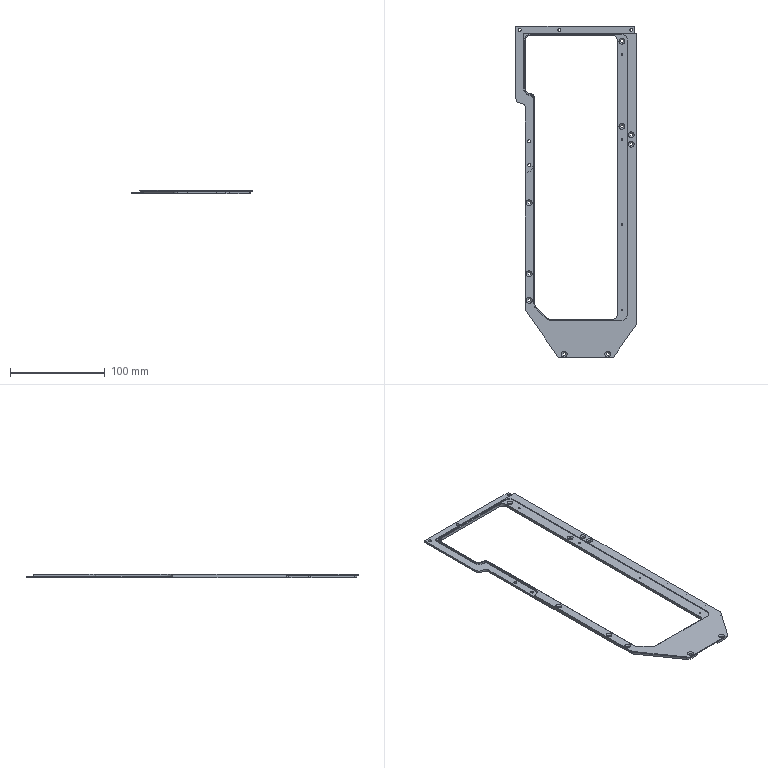NC program | NX | posted with a generic post | part box 127 x 351 x 4 mm
Whole program:
N10 G17 G21 G94 G90
(SPOT_FACING , TOOL : CHAMFER_D8-90DEG)
N12 T01 M6
N14 G54
N16 G17 G0 G90 X153.952 Y40.61 S2500 M3
N18 G43 Z20. H1
N20 G94 G82 G99 Z-2.5 F200. P200 R6.
N22 Y-28.911
N24 G80
N26 G0 X153.952 Y-28.911 Z20.
(SPOT_FACING_COPY_1 , TOOL : CHAMFER_D8-90DEG)
N28 X-8. Y49.5
N30 G82 Z-1.5 F200. P200 R6.
N32 X-83.
N34 X-111.
N36 X-168. Y12.5
N38 Y-33.5
N40 X54. Y-58.5
N42 X163. Y-48.5
N44 X175. Y59.5
N46 Y-58.5
N48 G80
N50 G0 X175. Y-58.5 Z20.
N52 M5
(SPOT_FACING_COPY_1_COPY , TOOL : D2.5)
N54 T15 M6
N56 G54
N58 G17 G0 G90 X-8. Y49.5 S3000 M3
N60 G43 Z20. H15
N62 G94 G83 G99 Z-10. F200. Q2. R6.
N64 X-83.
N66 X-111.
N68 X-168. Y12.5
N70 Y-33.5
N72 X54. Y-58.5
N74 X175. Y59.5
N76 Y-58.5
N78 G80
N80 G0 X175. Y-58.5 Z20.
N82 M5
(SPOT_FACING_COPY , TOOL : DRILL_D4.3-54-83)
N84 T10 M6
N86 G54
N88 G17 G0 G90 X153.952 Y40.61 S3000 M3
N90 G43 Z20. H10
N92 G94 G83 G99 Z-15. F200. Q2. R6.
N94 Y-28.911
N96 G80
N98 G0 X153.952 Y-28.911 Z20.
N100 M5
(PLANAR_MILL_10 , TOOL : D6-18-D6-50-3T-ROUGH)
N102 T03 M6
N104 G54
N106 G17 G0 G90 X-99.149 Y-4.194 S4500 M3
N108 G43 Z20. H3
N110 Z2.
N112 G94 G1 X-99.14 Y-4.178 Z1.999 F800.
N114 X-99.028 Y-3.328 Z1.969
N116 X-99.285 Y-2.51 Z1.939
N118 X-99.865 Y-1.878 Z1.91
N120 X-100.657 Y-1.55 Z1.88
N122 X-101.343 Z1.856
N124 X-102.135 Y-1.878 Z1.826
N126 X-102.715 Y-2.51 Z1.796
N128 X-102.972 Y-3.328 Z1.766
N130 X-102.86 Y-4.178 Z1.736
N132 X-102.517 Y-4.772 Z1.712
N134 X-101.99 Y-5.215 Z1.688
N136 X-101.343 Y-5.45 Z1.664
N138 X-100.657 Z1.64
N140 X-100.01 Y-5.215 Z1.616
N142 X-99.483 Y-4.772 Z1.592
N144 X-99.14 Y-4.178 Z1.568
N146 X-99.028 Y-3.328 Z1.538
N148 X-99.285 Y-2.51 Z1.508
N150 X-99.865 Y-1.878 Z1.478
N152 X-100.657 Y-1.55 Z1.448
N154 X-101.343 Z1.424
N156 X-102.135 Y-1.878 Z1.394
N158 X-102.715 Y-2.51 Z1.364
N160 X-102.972 Y-3.328 Z1.334
N162 X-102.86 Y-4.178 Z1.304
N164 X-102.517 Y-4.772 Z1.28
N166 X-101.99 Y-5.215 Z1.256
N168 X-101.343 Y-5.45 Z1.232
N170 X-100.657 Z1.208
N172 X-100.01 Y-5.215 Z1.184
N174 X-99.483 Y-4.772 Z1.16
N176 X-99.14 Y-4.178 Z1.136
N178 X-99.028 Y-3.328 Z1.106
N180 X-99.285 Y-2.51 Z1.076
N182 X-99.865 Y-1.878 Z1.046
N184 X-100.657 Y-1.55 Z1.017
N186 X-101.343 Z0.993
N188 X-102.135 Y-1.878 Z0.963
N190 X-102.715 Y-2.51 Z0.933
N192 X-102.972 Y-3.328 Z0.903
N194 X-102.86 Y-4.178 Z0.873
N196 X-102.517 Y-4.772 Z0.849
N198 X-101.99 Y-5.215 Z0.825
N200 X-101.343 Y-5.45 Z0.801
N202 X-100.657 Z0.777
N204 X-100.01 Y-5.215 Z0.753
N206 X-99.483 Y-4.772 Z0.729
N208 X-99.14 Y-4.178 Z0.705
N210 X-99.028 Y-3.328 Z0.675
N212 X-99.285 Y-2.51 Z0.645
N214 X-99.865 Y-1.878 Z0.615
N216 X-100.657 Y-1.55 Z0.585
N218 X-101.343 Z0.561
N220 X-102.135 Y-1.878 Z0.531
N222 X-102.715 Y-2.51 Z0.501
N224 X-102.972 Y-3.328 Z0.471
N226 X-102.86 Y-4.178 Z0.441
N228 X-102.517 Y-4.772 Z0.417
N230 X-101.99 Y-5.215 Z0.393
N232 X-101.343 Y-5.45 Z0.369
N234 X-100.657 Z0.345
N236 X-100.01 Y-5.215 Z0.321
N238 X-99.483 Y-4.772 Z0.297
N240 X-99.14 Y-4.178 Z0.273
N242 X-99.028 Y-3.328 Z0.243
N244 X-99.285 Y-2.51 Z0.213
N246 X-99.865 Y-1.878 Z0.183
N248 X-100.657 Y-1.55 Z0.153
N250 X-101.343 Z0.129
N252 X-102.135 Y-1.878 Z0.099
N254 X-102.715 Y-2.51 Z0.07
N256 X-102.972 Y-3.328 Z0.04
N258 X-102.86 Y-4.178 Z0.01
N260 X-102.517 Y-4.772 Z-0.014
N262 X-101.99 Y-5.215 Z-0.038
N264 X-101.343 Y-5.45 Z-0.062
N266 X-100.657 Z-0.086
N268 X-100.01 Y-5.215 Z-0.11
N270 X-99.483 Y-4.772 Z-0.134
N272 X-99.14 Y-4.178 Z-0.158
N274 X-99.028 Y-3.328 Z-0.188
N276 X-99.285 Y-2.51 Z-0.218
N278 X-99.865 Y-1.878 Z-0.248
N280 X-100.657 Y-1.55 Z-0.278
N282 X-101.343 Z-0.302
N284 X-102.135 Y-1.878 Z-0.332
N286 X-102.715 Y-2.51 Z-0.362
N288 X-102.972 Y-3.328 Z-0.392
N290 X-102.86 Y-4.178 Z-0.422
N292 X-102.517 Y-4.772 Z-0.446
N294 X-101.99 Y-5.215 Z-0.47
N296 X-101.343 Y-5.45 Z-0.494
N298 X-100.657 Z-0.518
N300 X-100.01 Y-5.215 Z-0.542
N302 X-99.483 Y-4.772 Z-0.566
N304 X-99.14 Y-4.178 Z-0.59
N306 X-99.028 Y-3.328 Z-0.62
N308 X-99.285 Y-2.51 Z-0.65
N310 X-99.865 Y-1.878 Z-0.68
N312 X-100.657 Y-1.55 Z-0.71
N314 X-101.343 Z-0.734
N316 X-102.135 Y-1.878 Z-0.764
N318 X-102.715 Y-2.51 Z-0.794
N320 X-102.972 Y-3.328 Z-0.823
N322 X-102.86 Y-4.178 Z-0.853
N324 X-102.517 Y-4.772 Z-0.877
N326 X-101.99 Y-5.215 Z-0.901
N328 X-101.343 Y-5.45 Z-0.925
N330 X-100.657 Z-0.949
N332 X-100.01 Y-5.215 Z-0.973
N334 X-99.483 Y-4.772 Z-0.998
N336 X-99.14 Y-4.178 Z-1.021
N338 X-99.028 Y-3.328 Z-1.051
N340 X-99.285 Y-2.51 Z-1.081
N342 X-99.865 Y-1.878 Z-1.111
N344 X-100.657 Y-1.55 Z-1.141
N346 X-101.343 Z-1.165
N348 X-102.135 Y-1.878 Z-1.195
N350 X-102.715 Y-2.51 Z-1.225
N352 X-102.972 Y-3.328 Z-1.255
N354 X-102.86 Y-4.178 Z-1.285
N356 X-102.517 Y-4.772 Z-1.309
N358 X-101.99 Y-5.215 Z-1.333
N360 X-101.343 Y-5.45 Z-1.357
N362 X-100.657 Z-1.381
N364 X-100.01 Y-5.215 Z-1.405
N366 X-99.483 Y-4.772 Z-1.429
N368 X-99.14 Y-4.178 Z-1.453
N370 X-99.028 Y-3.328 Z-1.483
N372 X-99.285 Y-2.51 Z-1.513
N374 X-99.865 Y-1.878 Z-1.543
N376 X-100.657 Y-1.55 Z-1.573
N378 X-101.343 Z-1.597
N380 X-102.135 Y-1.878 Z-1.627
N382 X-102.715 Y-2.51 Z-1.657
N384 X-102.972 Y-3.328 Z-1.687
N386 X-102.86 Y-4.178 Z-1.717
N388 X-102.517 Y-4.772 Z-1.741
N390 X-101.99 Y-5.215 Z-1.765
N392 X-101.343 Y-5.45 Z-1.789
N394 X-100.657 Z-1.813
N396 X-100.01 Y-5.215 Z-1.837
N398 X-99.483 Y-4.772 Z-1.861
N400 X-99.14 Y-4.178 Z-1.885
N402 X-99.028 Y-3.328 Z-1.915
N404 X-99.285 Y-2.51 Z-1.944
N406 X-99.865 Y-1.878 Z-1.974
N408 X-100.657 Y-1.55 Z-2.004
N410 X-101.343 Z-2.028
N412 X-102.135 Y-1.878 Z-2.058
N414 X-102.715 Y-2.51 Z-2.088
N416 X-102.972 Y-3.328 Z-2.118
N418 X-102.86 Y-4.178 Z-2.148
N420 X-102.517 Y-4.772 Z-2.172
N422 X-101.99 Y-5.215 Z-2.196
N424 X-101.343 Y-5.45 Z-2.22
N426 X-100.657 Z-2.244
N428 X-100.01 Y-5.215 Z-2.268
N430 X-99.483 Y-4.772 Z-2.292
N432 X-99.14 Y-4.178 Z-2.316
N434 X-99.028 Y-3.328 Z-2.346
N436 X-99.285 Y-2.51 Z-2.376
N438 X-99.865 Y-1.878 Z-2.406
N440 X-100.657 Y-1.55 Z-2.436
N442 X-101.343 Z-2.46
N444 X-102.135 Y-1.878 Z-2.49
N446 X-102.715 Y-2.51 Z-2.52
N448 X-102.972 Y-3.328 Z-2.55
N450 X-102.86 Y-4.178 Z-2.58
N452 X-102.517 Y-4.772 Z-2.604
N454 X-101.99 Y-5.215 Z-2.628
N456 X-101.343 Y-5.45 Z-2.652
N458 X-100.657 Z-2.676
N460 X-100.01 Y-5.215 Z-2.7
N462 X-99.483 Y-4.772 Z-2.724
N464 X-99.14 Y-4.178 Z-2.748
N466 X-99.028 Y-3.328 Z-2.778
N468 X-99.285 Y-2.51 Z-2.808
N470 X-99.865 Y-1.878 Z-2.838
N472 X-100.657 Y-1.55 Z-2.867
N474 X-101.343 Z-2.891
N476 X-102.135 Y-1.878 Z-2.921
N478 X-102.715 Y-2.51 Z-2.951
N480 X-102.972 Y-3.328 Z-2.981
N482 X-102.86 Y-4.178 Z-3.011
N484 X-102.517 Y-4.772 Z-3.035
N486 X-101.99 Y-5.215 Z-3.059
N488 X-101.343 Y-5.45 Z-3.083
N490 X-100.657 Z-3.107
N492 X-100.01 Y-5.215 Z-3.131
N494 X-99.483 Y-4.772 Z-3.155
N496 X-99.14 Y-4.178 Z-3.179
N498 X-99.028 Y-3.328 Z-3.209
N500 X-99.285 Y-2.51 Z-3.239
N502 X-99.865 Y-1.878 Z-3.269
N504 X-100.657 Y-1.55 Z-3.299
N506 X-101.343 Z-3.323
N508 X-102.135 Y-1.878 Z-3.353
N510 X-102.715 Y-2.51 Z-3.383
N512 X-102.972 Y-3.328 Z-3.413
N514 X-102.86 Y-4.178 Z-3.443
N516 X-102.517 Y-4.772 Z-3.467
N518 X-101.99 Y-5.215 Z-3.491
N520 X-101.343 Y-5.45 Z-3.515
N522 X-100.657 Z-3.539
N524 X-100.01 Y-5.215 Z-3.563
N526 X-99.483 Y-4.772 Z-3.587
N528 X-99.14 Y-4.178 Z-3.611
N530 X-99.028 Y-3.328 Z-3.641
N532 X-99.285 Y-2.51 Z-3.671
N534 X-99.865 Y-1.878 Z-3.701
N536 X-100.657 Y-1.55 Z-3.731
N538 X-101.343 Z-3.755
N540 X-102.135 Y-1.878 Z-3.784
N542 X-102.715 Y-2.51 Z-3.814
N544 X-102.972 Y-3.328 Z-3.844
N546 X-102.86 Y-4.178 Z-3.874
N548 X-102.517 Y-4.772 Z-3.898
N550 X-101.99 Y-5.215 Z-3.922
N552 X-101.343 Y-5.45 Z-3.946
N554 X-100.657 Z-3.97
N556 X-100.01 Y-5.215 Z-3.994
N558 X-99.483 Y-4.772 Z-4.018
N560 X-99.14 Y-4.178 Z-4.042
N562 X-99.028 Y-3.328 Z-4.072
N564 X-99.285 Y-2.51 Z-4.102
N566 X-99.865 Y-1.878 Z-4.132
N568 X-100.657 Y-1.55 Z-4.162
N570 X-101.343 Z-4.186
N572 X-102.135 Y-1.878 Z-4.216
N574 X-102.715 Y-2.51 Z-4.246
N576 X-102.972 Y-3.328 Z-4.276
N578 X-102.86 Y-4.178 Z-4.306
N580 X-102.517 Y-4.772 Z-4.33
N582 X-101.99 Y-5.215 Z-4.354
N584 X-101.343 Y-5.45 Z-4.378
N586 X-100.657 Z-4.402
N588 X-100.01 Y-5.215 Z-4.426
N590 X-99.483 Y-4.772 Z-4.45
N592 X-99.14 Y-4.178 Z-4.474
N594 X-99.028 Y-3.328 Z-4.504
N596 X-99.285 Y-2.51 Z-4.534
N598 X-99.865 Y-1.878 Z-4.564
N600 X-100.657 Y-1.55 Z-4.594
N602 X-101.343 Z-4.618
N604 X-102.135 Y-1.878 Z-4.648
N606 X-102.715 Y-2.51 Z-4.677
N608 X-102.972 Y-3.328 Z-4.707
N610 X-102.86 Y-4.178 Z-4.737
N612 X-102.517 Y-4.772 Z-4.761
N614 X-101.99 Y-5.215 Z-4.785
N616 X-101.343 Y-5.45 Z-4.809
N618 X-100.657 Z-4.833
N620 X-100.01 Y-5.215 Z-4.857
N622 X-99.483 Y-4.772 Z-4.881
N624 X-99.14 Y-4.178 Z-4.905
N626 X-99.028 Y-3.328 Z-4.935
N628 X-99.285 Y-2.51 Z-4.965
N630 X-99.865 Y-1.878 Z-4.995
N632 X-100.657 Y-1.55 Z-5.025
N634 X-101.343 Z-5.049
N636 X-102.135 Y-1.878 Z-5.079
N638 X-102.715 Y-2.51 Z-5.109
N640 X-102.972 Y-3.328 Z-5.139
N642 X-102.86 Y-4.178 Z-5.169
N644 X-102.517 Y-4.772 Z-5.193
N646 X-101.99 Y-5.215 Z-5.217
N648 X-101.343 Y-5.45 Z-5.241
N650 X-100.657 Z-5.265
N652 X-100.01 Y-5.215 Z-5.289
N654 X-99.483 Y-4.772 Z-5.313
N656 X-99.14 Y-4.178 Z-5.337
N658 X-99.028 Y-3.328 Z-5.367
N660 X-99.285 Y-2.51 Z-5.397
N662 X-99.865 Y-1.878 Z-5.427
N664 X-100.657 Y-1.55 Z-5.457
N666 X-101.343 Z-5.481
N668 X-102.135 Y-1.878 Z-5.511
N670 X-102.715 Y-2.51 Z-5.541
N672 X-102.972 Y-3.328 Z-5.571
N674 X-102.86 Y-4.178 Z-5.6
N676 X-102.517 Y-4.772 Z-5.624
N678 X-101.99 Y-5.215 Z-5.648
N680 X-101.343 Y-5.45 Z-5.673
N682 X-100.657 Z-5.696
N684 X-100.01 Y-5.215 Z-5.721
N686 X-99.483 Y-4.772 Z-5.745
N688 X-99.14 Y-4.178 Z-5.769
N690 X-99.028 Y-3.328 Z-5.798
N692 X-99.285 Y-2.51 Z-5.828
N694 X-99.865 Y-1.878 Z-5.858
N696 X-100.657 Y-1.55 Z-5.888
N698 X-101.343 Z-5.912
N700 X-102.135 Y-1.878 Z-5.942
N702 X-102.715 Y-2.51 Z-5.972
N704 X-102.972 Y-3.328 Z-6.002
N706 X-102.86 Y-4.178 Z-6.032
N708 X-102.517 Y-4.772 Z-6.056
N710 X-101.99 Y-5.215 Z-6.08
N712 X-101.343 Y-5.45 Z-6.104
N714 X-100.657 Z-6.128
N716 X-100.01 Y-5.215 Z-6.152
N718 X-99.483 Y-4.772 Z-6.176
N720 X-99.14 Y-4.178 Z-6.2
N722 X-99.028 Y-3.328 Z-6.23
N724 X-99.285 Y-2.51 Z-6.26
N726 X-99.865 Y-1.878 Z-6.29
N728 X-100.657 Y-1.55 Z-6.32
N730 X-101.343 Z-6.344
N732 X-102.135 Y-1.878 Z-6.374
N734 X-102.715 Y-2.51 Z-6.404
N736 X-102.972 Y-3.328 Z-6.434
N738 X-102.86 Y-4.178 Z-6.464
N740 X-102.517 Y-4.772 Z-6.488
N742 X-101.99 Y-5.215 Z-6.512
N744 X-101.343 Y-5.45 Z-6.536
N746 X-100.657 Z-6.56
N748 X-100.01 Y-5.215 Z-6.584
N750 X-99.483 Y-4.772 Z-6.608
N752 X-99.14 Y-4.178 Z-6.632
N754 X-99.028 Y-3.328 Z-6.662
N756 X-99.285 Y-2.51 Z-6.692
N758 X-99.865 Y-1.878 Z-6.721
N760 X-100.657 Y-1.55 Z-6.751
N762 X-101.343 Z-6.775
N764 X-102.135 Y-1.878 Z-6.805
N766 X-102.715 Y-2.51 Z-6.835
N768 X-102.972 Y-3.328 Z-6.865
N770 X-102.86 Y-4.178 Z-6.895
N772 X-102.517 Y-4.772 Z-6.919
N774 X-101.99 Y-5.215 Z-6.943
N776 X-101.343 Y-5.45 Z-6.967
N778 X-100.657 Z-6.991
N780 X-100.01 Y-5.215 Z-7.015
N782 X-99.483 Y-4.772 Z-7.039
N784 X-99.14 Y-4.178 Z-7.063
N786 X-99.028 Y-3.328 Z-7.093
N788 X-99.285 Y-2.51 Z-7.123
N790 X-99.865 Y-1.878 Z-7.153
N792 X-100.657 Y-1.55 Z-7.183
N794 X-101.343 Z-7.207
N796 X-102.135 Y-1.878 Z-7.237
N798 X-102.715 Y-2.51 Z-7.267
N800 X-102.972 Y-3.328 Z-7.297
N802 X-102.86 Y-4.178 Z-7.327
N804 X-102.517 Y-4.772 Z-7.351
N806 X-101.99 Y-5.215 Z-7.375
N808 X-101.343 Y-5.45 Z-7.399
N810 X-100.657 Z-7.423
N812 X-100.01 Y-5.215 Z-7.447
N814 X-99.483 Y-4.772 Z-7.471
N816 X-99.14 Y-4.178 Z-7.495
N818 X-99.028 Y-3.328 Z-7.525
N820 X-99.285 Y-2.51 Z-7.555
N822 X-99.865 Y-1.878 Z-7.585
N824 X-100.657 Y-1.55 Z-7.614
N826 X-101.343 Z-7.638
N828 X-102.135 Y-1.878 Z-7.668
N830 X-102.715 Y-2.51 Z-7.698
N832 X-102.972 Y-3.328 Z-7.728
N834 X-102.86 Y-4.178 Z-7.758
N836 X-102.517 Y-4.772 Z-7.782
N838 X-101.99 Y-5.215 Z-7.806
N840 X-101.343 Y-5.45 Z-7.83
N842 X-100.657 Z-7.854
N844 X-100.01 Y-5.215 Z-7.878
N846 X-99.483 Y-4.772 Z-7.902
N848 X-99.14 Y-4.178 Z-7.926
N850 X-99.028 Y-3.328 Z-7.956
N852 X-99.285 Y-2.51 Z-7.986
N854 X-99.865 Y-1.878 Z-8.016
N856 X-100.657 Y-1.55 Z-8.046
N858 X-101.343 Z-8.07
N860 X-102.135 Y-1.878 Z-8.1
N862 X-102.715 Y-2.51 Z-8.13
N864 X-102.972 Y-3.328 Z-8.16
N866 X-102.86 Y-4.178 Z-8.19
N868 X-102.517 Y-4.772 Z-8.214
N870 X-101.99 Y-5.215 Z-8.238
N872 X-101.343 Y-5.45 Z-8.262
N874 X-100.657 Z-8.286
N876 X-100.01 Y-5.215 Z-8.31
N878 X-99.483 Y-4.772 Z-8.334
N880 X-99.14 Y-4.178 Z-8.358
N882 X-99.028 Y-3.328 Z-8.388
N884 X-99.285 Y-2.51 Z-8.418
N886 X-99.865 Y-1.878 Z-8.448
N888 X-100.657 Y-1.55 Z-8.478
N890 X-101.343 Z-8.502
N892 X-102.135 Y-1.878 Z-8.532
N894 X-102.715 Y-2.51 Z-8.561
N896 X-102.972 Y-3.328 Z-8.591
N898 X-102.86 Y-4.178 Z-8.621
N900 X-102.517 Y-4.772 Z-8.645
N902 X-101.99 Y-5.215 Z-8.669
N904 X-101.343 Y-5.45 Z-8.693
N906 X-100.657 Z-8.717
N908 X-100.01 Y-5.215 Z-8.741
N910 X-99.483 Y-4.772 Z-8.765
N912 X-99.14 Y-4.178 Z-8.789
N914 X-99.028 Y-3.328 Z-8.819
N916 X-99.285 Y-2.51 Z-8.849
N918 X-99.865 Y-1.878 Z-8.879
N920 X-100.657 Y-1.55 Z-8.909
N922 X-101.343 Z-8.933
N924 X-102.135 Y-1.878 Z-8.963
N926 X-102.715 Y-2.51 Z-8.993
N928 X-102.972 Y-3.328 Z-9.023
N930 X-102.86 Y-4.178 Z-9.053
N932 X-102.517 Y-4.772 Z-9.077
N934 X-101.99 Y-5.215 Z-9.101
N936 X-101.343 Y-5.45 Z-9.125
N938 X-100.657 Z-9.149
N940 X-100.01 Y-5.215 Z-9.173
N942 X-99.483 Y-4.772 Z-9.197
N944 X-99.14 Y-4.178 Z-9.221
N946 X-99.028 Y-3.328 Z-9.251
N948 X-99.285 Y-2.51 Z-9.281
N950 X-99.865 Y-1.878 Z-9.311
N952 X-100.657 Y-1.55 Z-9.341
N954 X-101.343 Z-9.365
N956 X-102.135 Y-1.878 Z-9.395
N958 X-102.715 Y-2.51 Z-9.425
N960 X-102.972 Y-3.328 Z-9.454
N962 X-102.86 Y-4.178 Z-9.484
N964 X-102.517 Y-4.772 Z-9.508
N966 X-101.99 Y-5.215 Z-9.532
N968 X-101.343 Y-5.45 Z-9.556
N970 X-100.657 Z-9.58
N972 X-100.01 Y-5.215 Z-9.604
N974 X-99.483 Y-4.772 Z-9.629
N976 X-99.14 Y-4.178 Z-9.652
N978 X-99.028 Y-3.328 Z-9.682
N980 X-99.285 Y-2.51 Z-9.712
N982 X-99.865 Y-1.878 Z-9.742
N984 X-100.657 Y-1.55 Z-9.772
N986 X-101.343 Z-9.796
N988 X-102.135 Y-1.878 Z-9.826
N990 X-102.715 Y-2.51 Z-9.856
N992 X-102.972 Y-3.328 Z-9.886
N994 X-102.86 Y-4.178 Z-9.916
N996 X-102.517 Y-4.772 Z-9.94
N998 X-101.99 Y-5.215 Z-9.964
N1000 X-101.343 Y-5.45 Z-9.988
N1002 X-101. Z-10.
N1004 G3 X-99.05 Y-3.5 R1.95
N1006 X-101. Y-5.45 R-1.95
N1008 G1 Z-8.
N1010 G0 Z20.
N1012 X120.851 Y-4.194
N1014 Z2.
N1016 G1 X120.86 Y-4.178 Z1.999
N1018 X120.972 Y-3.328 Z1.969
N1020 X120.715 Y-2.51 Z1.939
N1022 X120.135 Y-1.878 Z1.91
N1024 X119.343 Y-1.55 Z1.88
N1026 X118.657 Z1.856
N1028 X117.865 Y-1.878 Z1.826
N1030 X117.285 Y-2.51 Z1.796
N1032 X117.028 Y-3.328 Z1.766
N1034 X117.14 Y-4.178 Z1.736
N1036 X117.483 Y-4.772 Z1.712
N1038 X118.01 Y-5.215 Z1.688
N1040 X118.657 Y-5.45 Z1.664
N1042 X119.343 Z1.64
N1044 X119.99 Y-5.215 Z1.616
N1046 X120.517 Y-4.772 Z1.592
N1048 X120.86 Y-4.178 Z1.568
N1050 X120.972 Y-3.328 Z1.538
N1052 X120.715 Y-2.51 Z1.508
N1054 X120.135 Y-1.878 Z1.478
N1056 X119.343 Y-1.55 Z1.448
N1058 X118.657 Z1.424
N1060 X117.865 Y-1.878 Z1.394
N1062 X117.285 Y-2.51 Z1.364
N1064 X117.028 Y-3.328 Z1.334
N1066 X117.14 Y-4.178 Z1.304
N1068 X117.483 Y-4.772 Z1.28
N1070 X118.01 Y-5.215 Z1.256
N1072 X118.657 Y-5.45 Z1.232
N1074 X119.343 Z1.208
N1076 X119.99 Y-5.215 Z1.184
N1078 X120.517 Y-4.772 Z1.16
N1080 X120.86 Y-4.178 Z1.136
N1082 X120.972 Y-3.328 Z1.106
N1084 X120.715 Y-2.51 Z1.076
N1086 X120.135 Y-1.878 Z1.046
N1088 X119.343 Y-1.55 Z1.017
N1090 X118.657 Z0.993
N1092 X117.865 Y-1.878 Z0.963
N1094 X117.285 Y-2.51 Z0.933
N1096 X117.028 Y-3.328 Z0.903
N1098 X117.14 Y-4.178 Z0.873
N1100 X117.483 Y-4.772 Z0.849
N1102 X118.01 Y-5.215 Z0.825
N1104 X118.657 Y-5.45 Z0.801
N1106 X119.343 Z0.777
N1108 X119.99 Y-5.215 Z0.753
N1110 X120.517 Y-4.772 Z0.729
N1112 X120.86 Y-4.178 Z0.705
N1114 X120.972 Y-3.328 Z0.675
N1116 X120.715 Y-2.51 Z0.645
N1118 X120.135 Y-1.878 Z0.615
N1120 X119.343 Y-1.55 Z0.585
N1122 X118.657 Z0.561
N1124 X117.865 Y-1.878 Z0.531
N1126 X117.285 Y-2.51 Z0.501
N1128 X117.028 Y-3.328 Z0.471
N1130 X117.14 Y-4.178 Z0.441
N1132 X117.483 Y-4.772 Z0.417
N1134 X118.01 Y-5.215 Z0.393
N1136 X118.657 Y-5.45 Z0.369
N1138 X119.343 Z0.345
N1140 X119.99 Y-5.215 Z0.321
N1142 X120.517 Y-4.772 Z0.297
N1144 X120.86 Y-4.178 Z0.273
N1146 X120.972 Y-3.328 Z0.243
N1148 X120.715 Y-2.51 Z0.213
N1150 X120.135 Y-1.878 Z0.183
N1152 X119.343 Y-1.55 Z0.153
N1154 X118.657 Z0.129
N1156 X117.865 Y-1.878 Z0.099
N1158 X117.285 Y-2.51 Z0.07
N1160 X117.028 Y-3.328 Z0.04
N1162 X117.14 Y-4.178 Z0.01
N1164 X117.483 Y-4.772 Z-0.014
N1166 X118.01 Y-5.215 Z-0.038
N1168 X118.657 Y-5.45 Z-0.062
N1170 X119.343 Z-0.086
N1172 X119.99 Y-5.215 Z-0.11
N1174 X120.517 Y-4.772 Z-0.134
N1176 X120.86 Y-4.178 Z-0.158
N1178 X120.972 Y-3.328 Z-0.188
N1180 X120.715 Y-2.51 Z-0.218
N1182 X120.135 Y-1.878 Z-0.248
N1184 X119.343 Y-1.55 Z-0.278
N1186 X118.657 Z-0.302
N1188 X117.865 Y-1.878 Z-0.332
N1190 X117.285 Y-2.51 Z-0.362
N1192 X117.028 Y-3.328 Z-0.392
N1194 X117.14 Y-4.178 Z-0.422
N1196 X117.483 Y-4.772 Z-0.446
N1198 X118.01 Y-5.215 Z-0.47
N1200 X118.657 Y-5.45 Z-0.494
N1202 X119.343 Z-0.518
N1204 X119.99 Y-5.215 Z-0.542
N1206 X120.517 Y-4.772 Z-0.566
N1208 X120.86 Y-4.178 Z-0.59
N1210 X120.972 Y-3.328 Z-0.62
N1212 X120.715 Y-2.51 Z-0.65
N1214 X120.135 Y-1.878 Z-0.68
N1216 X119.343 Y-1.55 Z-0.71
N1218 X118.657 Z-0.734
N1220 X117.865 Y-1.878 Z-0.764
N1222 X117.285 Y-2.51 Z-0.794
N1224 X117.028 Y-3.328 Z-0.823
N1226 X117.14 Y-4.178 Z-0.853
N1228 X117.483 Y-4.772 Z-0.877
N1230 X118.01 Y-5.215 Z-0.901
N1232 X118.657 Y-5.45 Z-0.925
N1234 X119.343 Z-0.949
N1236 X119.99 Y-5.215 Z-0.973
N1238 X120.517 Y-4.772 Z-0.998
N1240 X120.86 Y-4.178 Z-1.021
N1242 X120.972 Y-3.328 Z-1.051
N1244 X120.715 Y-2.51 Z-1.081
N1246 X120.135 Y-1.878 Z-1.111
N1248 X119.343 Y-1.55 Z-1.141
N1250 X118.657 Z-1.165
N1252 X117.865 Y-1.878 Z-1.195
N1254 X117.285 Y-2.51 Z-1.225
N1256 X117.028 Y-3.328 Z-1.255
N1258 X117.14 Y-4.178 Z-1.285
N1260 X117.483 Y-4.772 Z-1.309
N1262 X118.01 Y-5.215 Z-1.333
N1264 X118.657 Y-5.45 Z-1.357
N1266 X119.343 Z-1.381
N1268 X119.99 Y-5.215 Z-1.405
N1270 X120.517 Y-4.772 Z-1.429
N1272 X120.86 Y-4.178 Z-1.453
N1274 X120.972 Y-3.328 Z-1.483
N1276 X120.715 Y-2.51 Z-1.513
N1278 X120.135 Y-1.878 Z-1.543
N1280 X119.343 Y-1.55 Z-1.573
N1282 X118.657 Z-1.597
N1284 X117.865 Y-1.878 Z-1.627
N1286 X117.285 Y-2.51 Z-1.657
N1288 X117.028 Y-3.328 Z-1.687
N1290 X117.14 Y-4.178 Z-1.717
N1292 X117.483 Y-4.772 Z-1.741
N1294 X118.01 Y-5.215 Z-1.765
N1296 X118.657 Y-5.45 Z-1.789
N1298 X119.343 Z-1.813
N1300 X119.99 Y-5.215 Z-1.837
N1302 X120.517 Y-4.772 Z-1.861
N1304 X120.86 Y-4.178 Z-1.885
N1306 X120.972 Y-3.328 Z-1.915
N1308 X120.715 Y-2.51 Z-1.944
N1310 X120.135 Y-1.878 Z-1.974
N1312 X119.343 Y-1.55 Z-2.004
N1314 X118.657 Z-2.028
N1316 X117.865 Y-1.878 Z-2.058
N1318 X117.285 Y-2.51 Z-2.088
N1320 X117.028 Y-3.328 Z-2.118
N1322 X117.14 Y-4.178 Z-2.148
N1324 X117.483 Y-4.772 Z-2.172
N1326 X118.01 Y-5.215 Z-2.196
N1328 X118.657 Y-5.45 Z-2.22
N1330 X119.343 Z-2.244
N1332 X119.99 Y-5.215 Z-2.268
N1334 X120.517 Y-4.772 Z-2.292
N1336 X120.86 Y-4.178 Z-2.316
N1338 X120.972 Y-3.328 Z-2.346
N1340 X120.715 Y-2.51 Z-2.376
N1342 X120.135 Y-1.878 Z-2.406
N1344 X119.343 Y-1.55 Z-2.436
N1346 X118.657 Z-2.46
N1348 X117.865 Y-1.878 Z-2.49
N1350 X117.285 Y-2.51 Z-2.52
N1352 X117.028 Y-3.328 Z-2.55
N1354 X117.14 Y-4.178 Z-2.58
N1356 X117.483 Y-4.772 Z-2.604
N1358 X118.01 Y-5.215 Z-2.628
N1360 X118.657 Y-5.45 Z-2.652
N1362 X119.343 Z-2.676
N1364 X119.99 Y-5.215 Z-2.7
N1366 X120.517 Y-4.772 Z-2.724
N1368 X120.86 Y-4.178 Z-2.748
N1370 X120.972 Y-3.328 Z-2.778
N1372 X120.715 Y-2.51 Z-2.808
N1374 X120.135 Y-1.878 Z-2.838
N1376 X119.343 Y-1.55 Z-2.867
N1378 X118.657 Z-2.891
N1380 X117.865 Y-1.878 Z-2.921
N1382 X117.285 Y-2.51 Z-2.951
N1384 X117.028 Y-3.328 Z-2.981
N1386 X117.14 Y-4.178 Z-3.011
N1388 X117.483 Y-4.772 Z-3.035
N1390 X118.01 Y-5.215 Z-3.059
N1392 X118.657 Y-5.45 Z-3.083
N1394 X119.343 Z-3.107
N1396 X119.99 Y-5.215 Z-3.131
N1398 X120.517 Y-4.772 Z-3.155
N1400 X120.86 Y-4.178 Z-3.179
N1402 X120.972 Y-3.328 Z-3.209
N1404 X120.715 Y-2.51 Z-3.239
N1406 X120.135 Y-1.878 Z-3.269
N1408 X119.343 Y-1.55 Z-3.299
N1410 X118.657 Z-3.323
N1412 X117.865 Y-1.878 Z-3.353
N1414 X117.285 Y-2.51 Z-3.383
N1416 X117.028 Y-3.328 Z-3.413
N1418 X117.14 Y-4.178 Z-3.443
N1420 X117.483 Y-4.772 Z-3.467
N1422 X118.01 Y-5.215 Z-3.491
N1424 X118.657 Y-5.45 Z-3.515
N1426 X119.343 Z-3.539
N1428 X119.99 Y-5.215 Z-3.563
N1430 X120.517 Y-4.772 Z-3.587
N1432 X120.86 Y-4.178 Z-3.611
N1434 X120.972 Y-3.328 Z-3.641
N1436 X120.715 Y-2.51 Z-3.671
N1438 X120.135 Y-1.878 Z-3.701
N1440 X119.343 Y-1.55 Z-3.731
N1442 X118.657 Z-3.755
N1444 X117.865 Y-1.878 Z-3.784
N1446 X117.285 Y-2.51 Z-3.814
N1448 X117.028 Y-3.328 Z-3.844
N1450 X117.14 Y-4.178 Z-3.874
N1452 X117.483 Y-4.772 Z-3.898
N1454 X118.01 Y-5.215 Z-3.922
N1456 X118.657 Y-5.45 Z-3.946
N1458 X119.343 Z-3.97
N1460 X119.99 Y-5.215 Z-3.994
N1462 X120.517 Y-4.772 Z-4.018
N1464 X120.86 Y-4.178 Z-4.042
N1466 X120.972 Y-3.328 Z-4.072
N1468 X120.715 Y-2.51 Z-4.102
N1470 X120.135 Y-1.878 Z-4.132
N1472 X119.343 Y-1.55 Z-4.162
N1474 X118.657 Z-4.186
N1476 X117.865 Y-1.878 Z-4.216
N1478 X117.285 Y-2.51 Z-4.246
N1480 X117.028 Y-3.328 Z-4.276
N1482 X117.14 Y-4.178 Z-4.306
N1484 X117.483 Y-4.772 Z-4.33
N1486 X118.01 Y-5.215 Z-4.354
N1488 X118.657 Y-5.45 Z-4.378
N1490 X119.343 Z-4.402
N1492 X119.99 Y-5.215 Z-4.426
N1494 X120.517 Y-4.772 Z-4.45
N1496 X120.86 Y-4.178 Z-4.474
N1498 X120.972 Y-3.328 Z-4.504
N1500 X120.715 Y-2.51 Z-4.534
N1502 X120.135 Y-1.878 Z-4.564
N1504 X119.343 Y-1.55 Z-4.594
N1506 X118.657 Z-4.618
N1508 X117.865 Y-1.878 Z-4.648
N1510 X117.285 Y-2.51 Z-4.677
N1512 X117.028 Y-3.328 Z-4.707
N1514 X117.14 Y-4.178 Z-4.737
N1516 X117.483 Y-4.772 Z-4.761
N1518 X118.01 Y-5.215 Z-4.785
N1520 X118.657 Y-5.45 Z-4.809
N1522 X119.343 Z-4.833
N1524 X119.99 Y-5.215 Z-4.857
N1526 X120.517 Y-4.772 Z-4.881
N1528 X120.86 Y-4.178 Z-4.905
N1530 X120.972 Y-3.328 Z-4.935
N1532 X120.715 Y-2.51 Z-4.965
N1534 X120.135 Y-1.878 Z-4.995
N1536 X119.343 Y-1.55 Z-5.025
N1538 X118.657 Z-5.049
N1540 X117.865 Y-1.878 Z-5.079
N1542 X117.285 Y-2.51 Z-5.109
N1544 X117.028 Y-3.328 Z-5.139
N1546 X117.14 Y-4.178 Z-5.169
N1548 X117.483 Y-4.772 Z-5.193
N1550 X118.01 Y-5.215 Z-5.217
N1552 X118.657 Y-5.45 Z-5.241
N1554 X119.343 Z-5.265
N1556 X119.99 Y-5.215 Z-5.289
N1558 X120.517 Y-4.772 Z-5.313
N1560 X120.86 Y-4.178 Z-5.337
N1562 X120.972 Y-3.328 Z-5.367
N1564 X120.715 Y-2.51 Z-5.397
N1566 X120.135 Y-1.878 Z-5.427
N1568 X119.343 Y-1.55 Z-5.457
N1570 X118.657 Z-5.481
N1572 X117.865 Y-1.878 Z-5.511
N1574 X117.285 Y-2.51 Z-5.541
N1576 X117.028 Y-3.328 Z-5.571
N1578 X117.14 Y-4.178 Z-5.6
N1580 X117.483 Y-4.772 Z-5.624
N1582 X118.01 Y-5.215 Z-5.648
N1584 X118.657 Y-5.45 Z-5.673
N1586 X119.343 Z-5.696
N1588 X119.99 Y-5.215 Z-5.721
N1590 X120.517 Y-4.772 Z-5.745
N1592 X120.86 Y-4.178 Z-5.769
N1594 X120.972 Y-3.328 Z-5.798
N1596 X120.715 Y-2.51 Z-5.828
N1598 X120.135 Y-1.878 Z-5.858
N1600 X119.343 Y-1.55 Z-5.888
N1602 X118.657 Z-5.912
N1604 X117.865 Y-1.878 Z-5.942
N1606 X117.285 Y-2.51 Z-5.972
N1608 X117.028 Y-3.328 Z-6.002
N1610 X117.14 Y-4.178 Z-6.032
N1612 X117.483 Y-4.772 Z-6.056
N1614 X118.01 Y-5.215 Z-6.08
N1616 X118.657 Y-5.45 Z-6.104
N1618 X119.343 Z-6.128
N1620 X119.99 Y-5.215 Z-6.152
N1622 X120.517 Y-4.772 Z-6.176
N1624 X120.86 Y-4.178 Z-6.2
N1626 X120.972 Y-3.328 Z-6.23
N1628 X120.715 Y-2.51 Z-6.26
N1630 X120.135 Y-1.878 Z-6.29
N1632 X119.343 Y-1.55 Z-6.32
N1634 X118.657 Z-6.344
N1636 X117.865 Y-1.878 Z-6.374
N1638 X117.285 Y-2.51 Z-6.404
N1640 X117.028 Y-3.328 Z-6.434
N1642 X117.14 Y-4.178 Z-6.464
N1644 X117.483 Y-4.772 Z-6.488
N1646 X118.01 Y-5.215 Z-6.512
N1648 X118.657 Y-5.45 Z-6.536
N1650 X119.343 Z-6.56
N1652 X119.99 Y-5.215 Z-6.584
N1654 X120.517 Y-4.772 Z-6.608
N1656 X120.86 Y-4.178 Z-6.632
N1658 X120.972 Y-3.328 Z-6.662
N1660 X120.715 Y-2.51 Z-6.692
N1662 X120.135 Y-1.878 Z-6.721
N1664 X119.343 Y-1.55 Z-6.751
N1666 X118.657 Z-6.775
N1668 X117.865 Y-1.878 Z-6.805
N1670 X117.285 Y-2.51 Z-6.835
N1672 X117.028 Y-3.328 Z-6.865
N1674 X117.14 Y-4.178 Z-6.895
N1676 X117.483 Y-4.772 Z-6.919
N1678 X118.01 Y-5.215 Z-6.943
N1680 X118.657 Y-5.45 Z-6.967
N1682 X119.343 Z-6.991
N1684 X119.99 Y-5.215 Z-7.015
N1686 X120.517 Y-4.772 Z-7.039
N1688 X120.86 Y-4.178 Z-7.063
N1690 X120.972 Y-3.328 Z-7.093
N1692 X120.715 Y-2.51 Z-7.123
N1694 X120.135 Y-1.878 Z-7.153
N1696 X119.343 Y-1.55 Z-7.183
N1698 X118.657 Z-7.207
N1700 X117.865 Y-1.878 Z-7.237
N1702 X117.285 Y-2.51 Z-7.267
N1704 X117.028 Y-3.328 Z-7.297
N1706 X117.14 Y-4.178 Z-7.327
N1708 X117.483 Y-4.772 Z-7.351
N1710 X118.01 Y-5.215 Z-7.375
N1712 X118.657 Y-5.45 Z-7.399
N1714 X119.343 Z-7.423
N1716 X119.99 Y-5.215 Z-7.447
N1718 X120.517 Y-4.772 Z-7.471
N1720 X120.86 Y-4.178 Z-7.495
N1722 X120.972 Y-3.328 Z-7.525
N1724 X120.715 Y-2.51 Z-7.555
N1726 X120.135 Y-1.878 Z-7.585
N1728 X119.343 Y-1.55 Z-7.614
N1730 X118.657 Z-7.638
N1732 X117.865 Y-1.878 Z-7.668
N1734 X117.285 Y-2.51 Z-7.698
N1736 X117.028 Y-3.328 Z-7.728
N1738 X117.14 Y-4.178 Z-7.758
N1740 X117.483 Y-4.772 Z-7.782
N1742 X118.01 Y-5.215 Z-7.806
N1744 X118.657 Y-5.45 Z-7.83
N1746 X119.343 Z-7.854
N1748 X119.99 Y-5.215 Z-7.878
N1750 X120.517 Y-4.772 Z-7.902
N1752 X120.86 Y-4.178 Z-7.926
N1754 X120.972 Y-3.328 Z-7.956
N1756 X120.715 Y-2.51 Z-7.986
N1758 X120.135 Y-1.878 Z-8.016
N1760 X119.343 Y-1.55 Z-8.046
N1762 X118.657 Z-8.07
N1764 X117.865 Y-1.878 Z-8.1
N1766 X117.285 Y-2.51 Z-8.13
N1768 X117.028 Y-3.328 Z-8.16
N1770 X117.14 Y-4.178 Z-8.19
N1772 X117.483 Y-4.772 Z-8.214
N1774 X118.01 Y-5.215 Z-8.238
N1776 X118.657 Y-5.45 Z-8.262
N1778 X119.343 Z-8.286
N1780 X119.99 Y-5.215 Z-8.31
N1782 X120.517 Y-4.772 Z-8.334
N1784 X120.86 Y-4.178 Z-8.358
N1786 X120.972 Y-3.328 Z-8.388
N1788 X120.715 Y-2.51 Z-8.418
N1790 X120.135 Y-1.878 Z-8.448
N1792 X119.343 Y-1.55 Z-8.478
N1794 X118.657 Z-8.502
N1796 X117.865 Y-1.878 Z-8.532
N1798 X117.285 Y-2.51 Z-8.561
N1800 X117.028 Y-3.328 Z-8.591
N1802 X117.14 Y-4.178 Z-8.621
N1804 X117.483 Y-4.772 Z-8.645
N1806 X118.01 Y-5.215 Z-8.669
N1808 X118.657 Y-5.45 Z-8.693
N1810 X119.343 Z-8.717
N1812 X119.99 Y-5.215 Z-8.741
N1814 X120.517 Y-4.772 Z-8.765
N1816 X120.86 Y-4.178 Z-8.789
N1818 X120.972 Y-3.328 Z-8.819
N1820 X120.715 Y-2.51 Z-8.849
N1822 X120.135 Y-1.878 Z-8.879
N1824 X119.343 Y-1.55 Z-8.909
N1826 X118.657 Z-8.933
N1828 X117.865 Y-1.878 Z-8.963
N1830 X117.285 Y-2.51 Z-8.993
N1832 X117.028 Y-3.328 Z-9.023
N1834 X117.14 Y-4.178 Z-9.053
N1836 X117.483 Y-4.772 Z-9.077
N1838 X118.01 Y-5.215 Z-9.101
N1840 X118.657 Y-5.45 Z-9.125
N1842 X119.343 Z-9.149
N1844 X119.99 Y-5.215 Z-9.173
N1846 X120.517 Y-4.772 Z-9.197
N1848 X120.86 Y-4.178 Z-9.221
N1850 X120.972 Y-3.328 Z-9.251
N1852 X120.715 Y-2.51 Z-9.281
N1854 X120.135 Y-1.878 Z-9.311
N1856 X119.343 Y-1.55 Z-9.341
N1858 X118.657 Z-9.365
N1860 X117.865 Y-1.878 Z-9.395
N1862 X117.285 Y-2.51 Z-9.425
N1864 X117.028 Y-3.328 Z-9.454
N1866 X117.14 Y-4.178 Z-9.484
N1868 X117.483 Y-4.772 Z-9.508
N1870 X118.01 Y-5.215 Z-9.532
N1872 X118.657 Y-5.45 Z-9.556
N1874 X119.343 Z-9.58
N1876 X119.99 Y-5.215 Z-9.604
N1878 X120.517 Y-4.772 Z-9.629
N1880 X120.86 Y-4.178 Z-9.652
N1882 X120.972 Y-3.328 Z-9.682
N1884 X120.715 Y-2.51 Z-9.712
N1886 X120.135 Y-1.878 Z-9.742
N1888 X119.343 Y-1.55 Z-9.772
N1890 X118.657 Z-9.796
N1892 X117.865 Y-1.878 Z-9.826
N1894 X117.285 Y-2.51 Z-9.856
N1896 X117.028 Y-3.328 Z-9.886
N1898 X117.14 Y-4.178 Z-9.916
N1900 X117.483 Y-4.772 Z-9.94
N1902 X118.01 Y-5.215 Z-9.964
N1904 X118.657 Y-5.45 Z-9.988
N1906 X119. Z-10.
N1908 G3 X120.95 Y-3.5 R1.95
N1910 X119. Y-5.45 R-1.95
N1912 G1 Z-8.
N1914 G0 Z20.
N1916 M5
(PLANAR_MILL_10_COPY , TOOL : D6-18-D6-50-3T-FINISH)
N1918 T04 M6
N1920 G54
N1922 G17 G0 G90 X-102. Y-3.5 S3500 M3
N1924 G43 Z20. H4
N1926 Z-8.
N1928 G94 G1 Z-10. F500.
N1930 Y-4.5
N1932 G3 X-101. Y-5.5 R1.
N1934 X-99. Y-3.5 R2.
N1936 X-101. Y-5.5 R-2.
N1938 X-100. Y-4.5 R1.
N1940 G1 Y-3.501
N1942 Z-8.
N1944 G0 Z20.
N1946 X118. Y-3.5
N1948 Z-8.
N1950 G1 Z-10.
N1952 Y-4.5
N1954 G3 X119. Y-5.5 R1.
N1956 X121. Y-3.5 R2.
N1958 X119. Y-5.5 R-2.
N1960 X120. Y-4.5 R1.
N1962 G1 Y-3.501
N1964 Z-8.
N1966 G0 Z20.
N1968 M5
(PLANAR_MILL_10_COPY_1 , TOOL : D6-18-D6-50-3T-ROUGH)
N1970 T03 M6
N1972 G54
N1974 G17 G0 G90 X-108.891 Y-5.181 S4500 M3
N1976 G43 Z20. H3
N1978 Z2.
N1980 G94 G1 X-108.923 Y-5.083 Z1.996 F800.
N1982 X-109.072 Y-3.152 Z1.929
N1984 X-108.758 Y-1.241 Z1.861
N1986 X-107.997 Y0.54 Z1.794
N1988 X-106.835 Y2.089 Z1.726
N1990 X-105.338 Y3.317 Z1.658
N1992 X-103.591 Y4.153 Z1.591
N1994 X-101.696 Y4.55 Z1.523
N1996 X-100.304 Z1.474
N1998 X-98.409 Y4.153 Z1.407
N2000 X-96.662 Y3.317 Z1.339
N2002 X-95.165 Y2.089 Z1.272
N2004 X-94.003 Y0.54 Z1.204
N2006 X-93.242 Y-1.241 Z1.136
N2008 X-92.928 Y-3.152 Z1.069
N2010 X-93.077 Y-5.083 Z1.001
N2012 X-93.681 Y-6.923 Z0.933
N2014 X-94.376 Y-8.127 Z0.885
N2016 X-95.538 Y-9.454 Z0.823
N2018 X-96.96 Y-10.497 Z0.762
N2020 X-98.574 Y-11.207 Z0.7
N2022 X-100.304 Y-11.55 Z0.638
N2024 X-101.696 Z0.59
N2026 X-103.426 Y-11.207 Z0.528
N2028 X-105.04 Y-10.497 Z0.467
N2030 X-106.462 Y-9.454 Z0.405
N2032 X-107.624 Y-8.127 Z0.344
N2034 X-108.319 Y-6.923 Z0.295
N2036 X-108.923 Y-5.083 Z0.227
N2038 X-109.072 Y-3.152 Z0.16
N2040 X-108.758 Y-1.241 Z0.092
N2042 X-107.997 Y0.54 Z0.024
N2044 X-106.835 Y2.089 Z-0.043
N2046 X-105.338 Y3.317 Z-0.111
N2048 X-103.591 Y4.153 Z-0.178
N2050 X-101.696 Y4.55 Z-0.246
N2052 X-100.304 Z-0.295
N2054 X-98.409 Y4.153 Z-0.362
N2056 X-96.662 Y3.317 Z-0.43
N2058 X-95.165 Y2.089 Z-0.497
N2060 X-94.003 Y0.54 Z-0.565
N2062 X-93.242 Y-1.241 Z-0.633
N2064 X-92.928 Y-3.152 Z-0.7
N2066 X-93.077 Y-5.083 Z-0.768
N2068 X-93.681 Y-6.923 Z-0.836
N2070 X-94.376 Y-8.127 Z-0.884
N2072 X-95.538 Y-9.454 Z-0.946
N2074 X-96.96 Y-10.497 Z-1.007
N2076 X-98.574 Y-11.207 Z-1.069
N2078 X-100.304 Y-11.55 Z-1.131
N2080 X-101.696 Z-1.179
N2082 X-103.426 Y-11.207 Z-1.241
N2084 X-105.04 Y-10.497 Z-1.302
N2086 X-106.462 Y-9.454 Z-1.364
N2088 X-107.624 Y-8.127 Z-1.425
N2090 X-108.319 Y-6.923 Z-1.474
N2092 X-108.923 Y-5.083 Z-1.542
N2094 X-109.072 Y-3.152 Z-1.609
N2096 X-108.758 Y-1.241 Z-1.677
N2098 X-107.997 Y0.54 Z-1.745
N2100 X-106.835 Y2.089 Z-1.812
N2102 X-105.338 Y3.317 Z-1.88
N2104 X-103.591 Y4.153 Z-1.947
N2106 X-101.696 Y4.55 Z-2.015
N2108 X-100.304 Z-2.064
N2110 X-98.409 Y4.153 Z-2.131
N2112 X-96.662 Y3.317 Z-2.199
N2114 X-95.165 Y2.089 Z-2.267
N2116 X-94.003 Y0.54 Z-2.334
N2118 X-93.242 Y-1.241 Z-2.402
N2120 X-92.928 Y-3.152 Z-2.469
N2122 X-93.077 Y-5.083 Z-2.537
N2124 X-93.681 Y-6.923 Z-2.605
N2126 X-94.376 Y-8.127 Z-2.653
N2128 X-95.538 Y-9.454 Z-2.715
N2130 X-96.96 Y-10.497 Z-2.776
N2132 X-98.574 Y-11.207 Z-2.838
N2134 X-100.304 Y-11.55 Z-2.9
N2136 X-101.696 Z-2.948
N2138 X-103.426 Y-11.207 Z-3.01
N2140 X-105.04 Y-10.497 Z-3.071
N2142 X-106.462 Y-9.454 Z-3.133
N2144 X-107.624 Y-8.127 Z-3.195
N2146 X-108.319 Y-6.923 Z-3.243
N2148 X-108.923 Y-5.083 Z-3.311
N2150 X-109.072 Y-3.152 Z-3.378
N2152 X-108.758 Y-1.241 Z-3.446
N2154 X-107.997 Y0.54 Z-3.514
N2156 X-106.835 Y2.089 Z-3.581
N2158 X-105.338 Y3.317 Z-3.649
N2160 X-103.591 Y4.153 Z-3.716
N2162 X-101.696 Y4.55 Z-3.784
N2164 X-100.304 Z-3.833
N2166 X-98.409 Y4.153 Z-3.9
N2168 X-96.662 Y3.317 Z-3.968
N2170 X-95.165 Y2.089 Z-4.036
N2172 X-94.003 Y0.54 Z-4.103
N2174 X-93.242 Y-1.241 Z-4.171
N2176 X-92.928 Y-3.152 Z-4.238
N2178 X-93.077 Y-5.083 Z-4.306
N2180 X-93.681 Y-6.923 Z-4.374
N2182 X-94.376 Y-8.127 Z-4.422
N2184 X-95.538 Y-9.454 Z-4.484
N2186 X-96.96 Y-10.497 Z-4.545
N2188 X-98.574 Y-11.207 Z-4.607
N2190 X-100.304 Y-11.55 Z-4.669
N2192 X-101.696 Z-4.717
N2194 X-103.426 Y-11.207 Z-4.779
N2196 X-105.04 Y-10.497 Z-4.84
N2198 X-106.462 Y-9.454 Z-4.902
N2200 X-107.624 Y-8.127 Z-4.964
N2202 X-108.319 Y-6.923 Z-5.012
N2204 X-108.923 Y-5.083 Z-5.08
N2206 X-109.072 Y-3.152 Z-5.147
N2208 X-108.758 Y-1.241 Z-5.215
N2210 X-107.997 Y0.54 Z-5.283
N2212 X-106.835 Y2.089 Z-5.35
N2214 X-105.338 Y3.317 Z-5.418
N2216 X-103.591 Y4.153 Z-5.486
N2218 X-101.696 Y4.55 Z-5.553
N2220 X-100.304 Z-5.602
N2222 X-98.409 Y4.153 Z-5.669
N2224 X-96.662 Y3.317 Z-5.737
N2226 X-95.165 Y2.089 Z-5.805
N2228 X-94.003 Y0.54 Z-5.872
N2230 X-93.242 Y-1.241 Z-5.94
N2232 X-92.928 Y-3.152 Z-6.007
N2234 X-93.077 Y-5.083 Z-6.075
N2236 X-93.681 Y-6.923 Z-6.143
N2238 X-94.376 Y-8.127 Z-6.191
N2240 X-95.538 Y-9.454 Z-6.253
N2242 X-96.96 Y-10.497 Z-6.314
N2244 X-98.574 Y-11.207 Z-6.376
N2246 X-100.304 Y-11.55 Z-6.438
N2248 X-101.696 Z-6.486
N2250 X-103.426 Y-11.207 Z-6.548
N2252 X-105.04 Y-10.497 Z-6.609
N2254 X-106.462 Y-9.454 Z-6.671
N2256 X-107.624 Y-8.127 Z-6.733
N2258 X-108.319 Y-6.923 Z-6.781
N2260 X-108.923 Y-5.083 Z-6.849
N2262 X-109.072 Y-3.152 Z-6.916
N2264 X-108.758 Y-1.241 Z-6.984
N2266 X-107.997 Y0.54 Z-7.052
N2268 X-106.835 Y2.089 Z-7.119
N2270 X-105.338 Y3.317 Z-7.187
N2272 X-103.591 Y4.153 Z-7.255
N2274 X-101.696 Y4.55 Z-7.322
N2276 X-100.304 Z-7.371
N2278 X-98.409 Y4.153 Z-7.438
N2280 X-96.662 Y3.317 Z-7.506
N2282 X-95.165 Y2.089 Z-7.574
N2284 X-94.003 Y0.54 Z-7.641
N2286 X-93.242 Y-1.241 Z-7.709
N2288 X-92.928 Y-3.152 Z-7.777
N2290 X-93.077 Y-5.083 Z-7.844
N2292 X-93.681 Y-6.923 Z-7.912
N2294 X-94.376 Y-8.127 Z-7.96
N2296 X-95.538 Y-9.454 Z-8.022
N2298 X-96.96 Y-10.497 Z-8.084
N2300 X-98.574 Y-11.207 Z-8.145
N2302 X-100.304 Y-11.55 Z-8.207
N2304 X-101.696 Z-8.255
N2306 X-103.426 Y-11.207 Z-8.317
N2308 X-105.04 Y-10.497 Z-8.378
N2310 X-106.462 Y-9.454 Z-8.44
N2312 X-107.624 Y-8.127 Z-8.502
N2314 X-108.319 Y-6.923 Z-8.55
N2316 X-108.923 Y-5.083 Z-8.618
N2318 X-109.072 Y-3.152 Z-8.685
N2320 X-108.758 Y-1.241 Z-8.753
N2322 X-107.997 Y0.54 Z-8.821
N2324 X-106.835 Y2.089 Z-8.888
N2326 X-105.338 Y3.317 Z-8.956
N2328 X-103.591 Y4.153 Z-9.024
N2330 X-101.696 Y4.55 Z-9.091
N2332 X-100.304 Z-9.14
N2334 X-98.409 Y4.153 Z-9.207
N2336 X-96.662 Y3.317 Z-9.275
N2338 X-95.165 Y2.089 Z-9.343
N2340 X-94.003 Y0.54 Z-9.41
N2342 X-93.242 Y-1.241 Z-9.478
N2344 X-92.928 Y-3.152 Z-9.546
N2346 X-93.077 Y-5.083 Z-9.613
N2348 X-93.681 Y-6.923 Z-9.681
N2350 X-94.376 Y-8.127 Z-9.729
N2352 X-95.538 Y-9.454 Z-9.791
N2354 X-96.96 Y-10.497 Z-9.853
N2356 X-98.574 Y-11.207 Z-9.914
N2358 X-100.304 Y-11.55 Z-9.976
N2360 X-101. Z-10.
N2362 G2 X-109.05 Y-3.5 R8.05
N2364 X-101. Y-11.55 R-8.05
N2366 G1 Z-8.
N2368 G0 Z20.
N2370 M5
(PLANAR_MILL_10_COPY_COPY , TOOL : D6-18-D6-50-3T-FINISH)
N2372 T04 M6
N2374 G54
N2376 G17 G0 G90 X-100. Y-12.5 S3500 M3
N2378 G43 Z20. H4
N2380 Z-8.
N2382 G94 G1 Z-10. F500.
N2384 G3 X-101. Y-11.5 R1.
N2386 G2 X-109. Y-3.5 R8.
N2388 X-101. Y-11.5 R-8.
N2390 G3 X-102. Y-12.5 R1.
N2392 G1 Z-8.
N2394 G0 Z20.
N2396 M5
N2398 M2